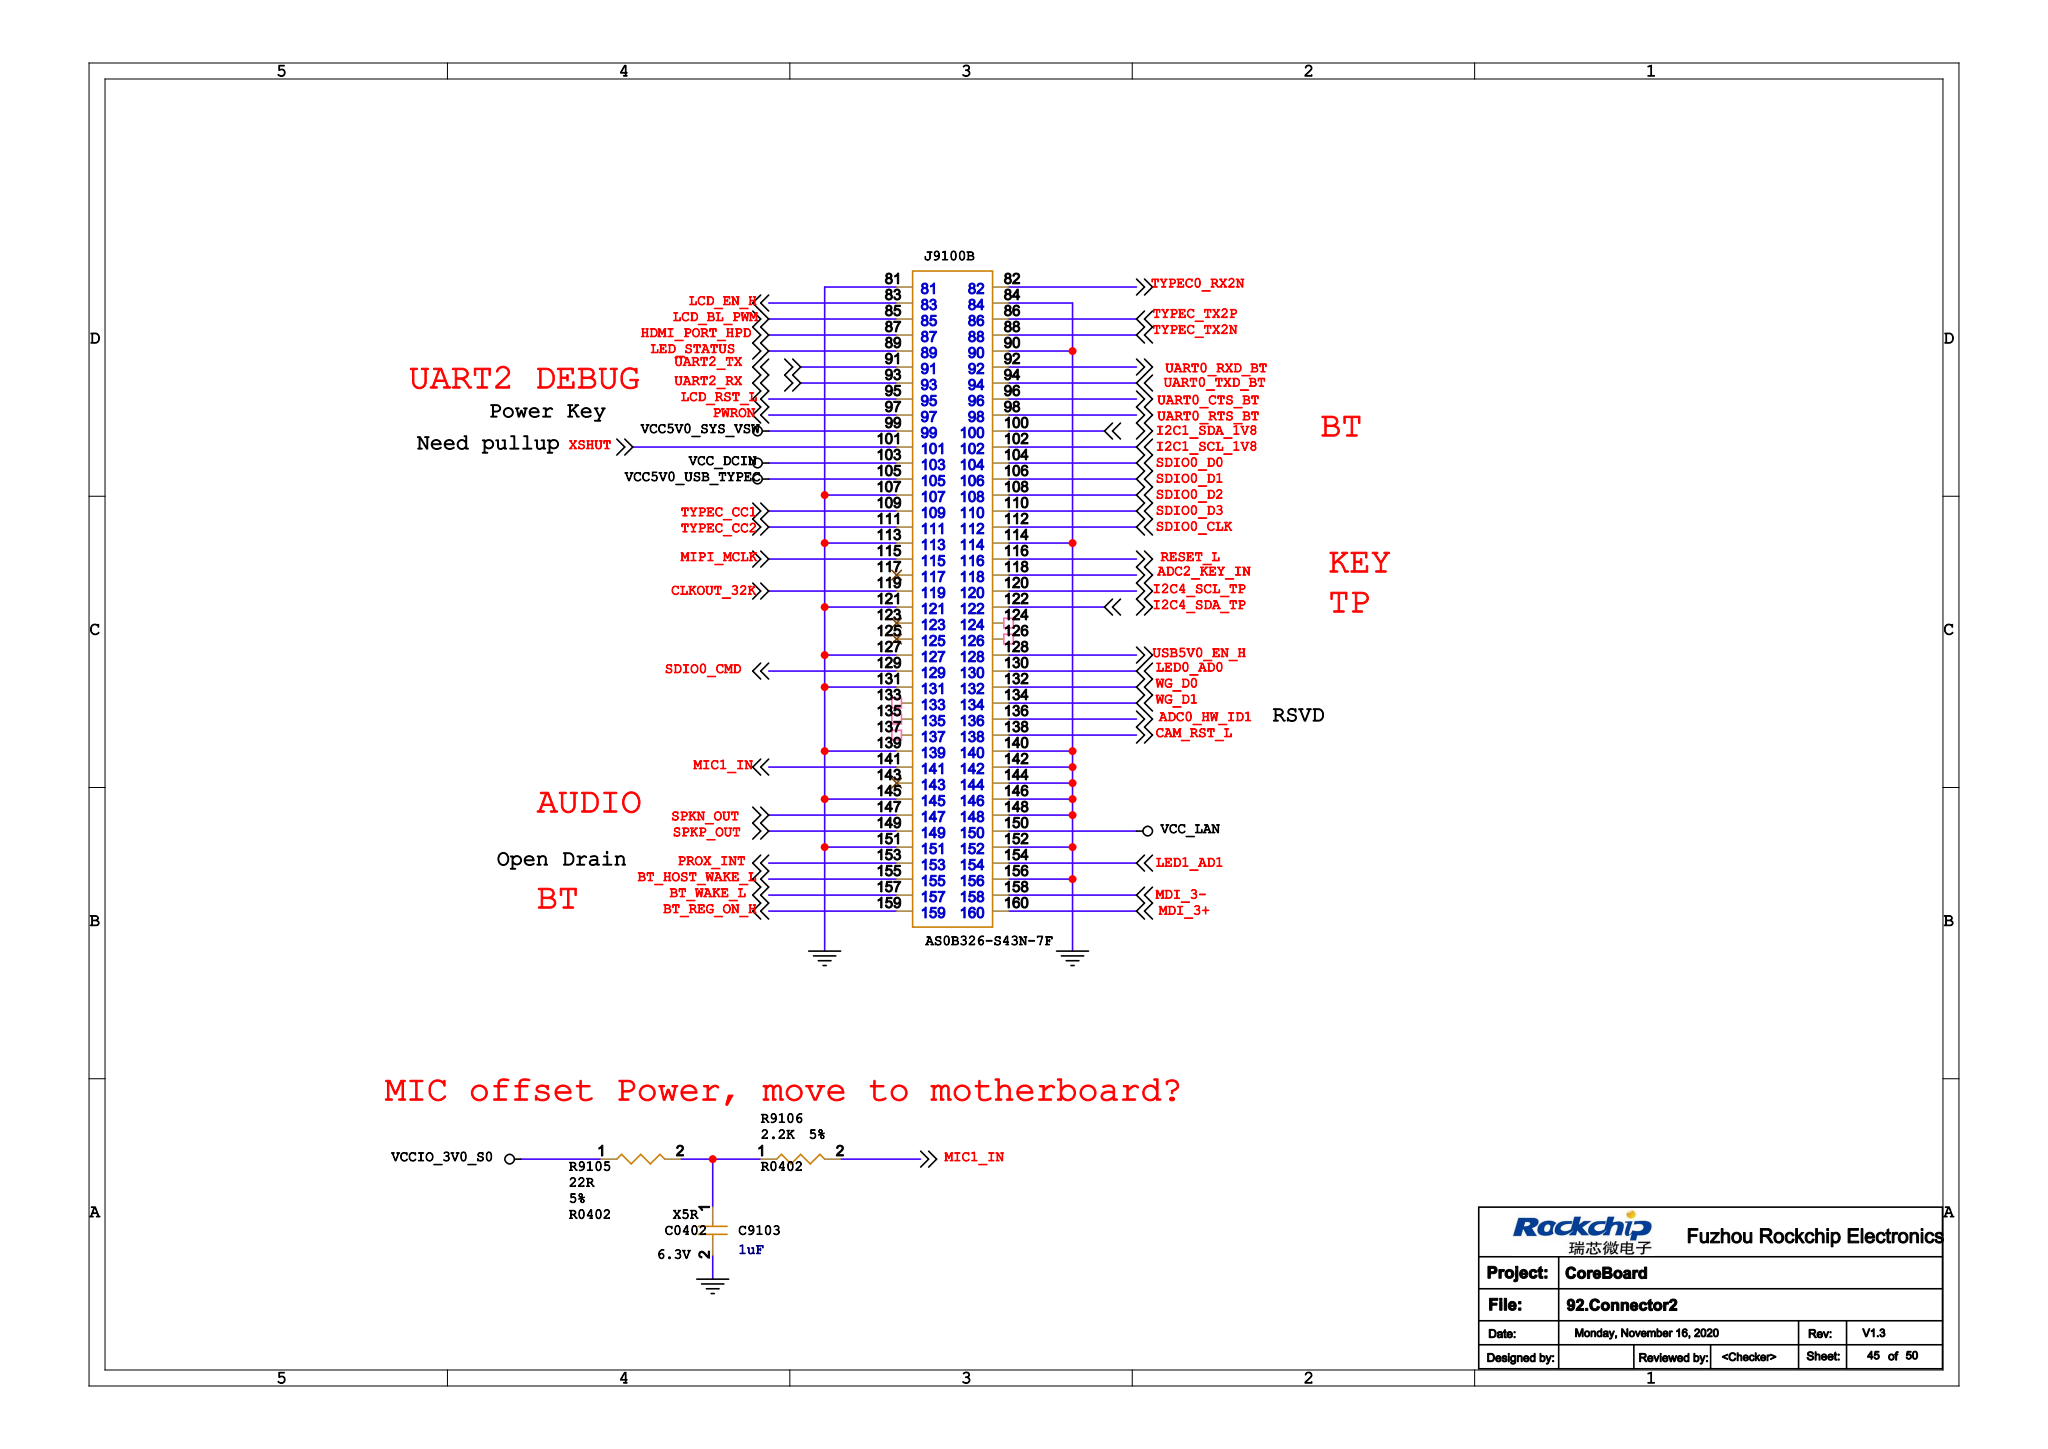Circuit board | Cadence Allegro | 749 parts | 717 nets | one sheet of the schematic
Parts on this sheet (reference | value | footprint):
C9103 | 1uF | C0402
J9100 | AS0B326-S43N-7F | MXM_230P_0P5
R9105 | 22R | R0402
R9106 | 2.2K | R0402
Nets of these parts (net: part-pin ...):
GND: C9103-2 J9100-5 J9100-81 J9100-84 J9100-90 J9100-107 J9100-113 J9100-114 J9100-121 J9100-127 J9100-131 J9100-139 J9100-140 J9100-142 J9100-144 J9100-145 J9100-146 J9100-148 J9100-151 J9100-152 J9100-156
TYPEC_CC1: J9100-109
TYPEC_CC2: J9100-111
I2C1_SDA_1V8: J9100-100
XSHUT: J9100-101
I2C1_SCL_1V8: J9100-102
VCC_DCIN: J9100-103
SDIO0_D0: J9100-104
VCC5V0_USB_TYPEC: J9100-105
SDIO0_D1: J9100-106
SDIO0_D2: J9100-108
SDIO0_D3: J9100-110
SDIO0_CLK: J9100-112
MIPI_MCLK: J9100-115
RESET_L: J9100-116
ADC2_KEY_IN: J9100-118
CLKOUT_32K: J9100-119
I2C4_SCL_TP: J9100-120
I2C4_SDA_TP: J9100-122
USB5V0_EN_H: J9100-128
SDIO0_CMD: J9100-129
LED0_AD0: J9100-130
WG_D0: J9100-132
WG_D1: J9100-134
ADC0_HW_ID1: J9100-136
CAM_RST_L: J9100-138
MIC1_IN: R9106-2 J9100-141
SPKN_OUT: J9100-147
SPKP_OUT: J9100-149
VCC_LAN: J9100-150
PROX_INT: J9100-153
LED1_AD1: J9100-154
BT_HOST_WAKE_L: J9100-155
BT_WAKE_L: J9100-157
MDI_3-: J9100-158
BT_REG_ON_H: J9100-159
MDI_3+: J9100-160
TYPEC0_RX2N: J9100-82
LCD_EN_H: J9100-83
LCD_BL_PWM: J9100-85
TYPEC_TX2P: J9100-86
HDMI_PORT_HPD: J9100-87
TYPEC_TX2N: J9100-88
LED_STATUS: J9100-89
UART2_TX: J9100-91
UART0_RXD_BT: J9100-92
UART2_RX: J9100-93
UART0_TXD_BT: J9100-94
LCD_RST_L: J9100-95
UART0_CTS_BT: J9100-96
PWRON: J9100-97
UART0_RTS_BT: J9100-98
VCC5V0_SYS_VSW: J9100-99
VCCIO_3V0_S0: R9105-1
N18728659: C9103-1 R9105-2 R9106-1